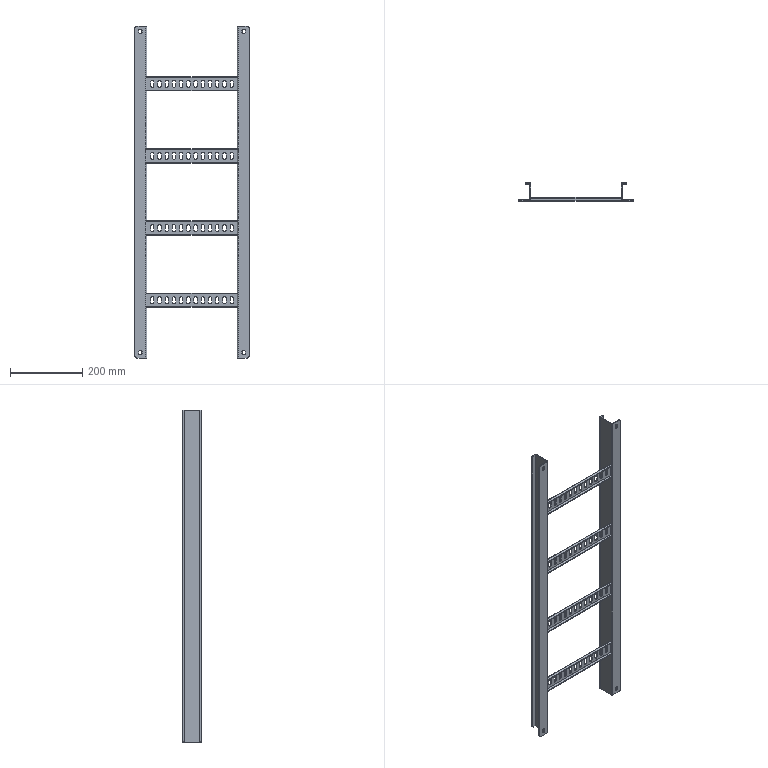Part | SolidWorks | 6 solids | 396 faces | box 316 x 50 x 920 mm | volume 614023 mm3 | plane 212 | cylinder 184 | commonest cylinder face diameters 9 x152 0.2 x12 5.2 x8 10 x8 6.2 x4